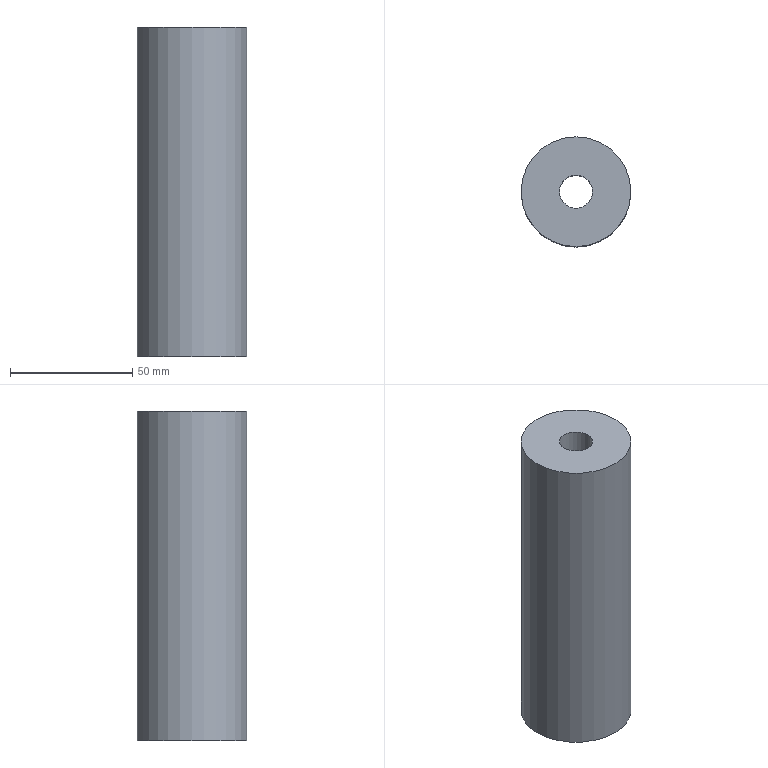Part | NX | features solid 2 | 1 solid | 6 faces | box 45 x 45 x 135.001 mm | volume 187665 mm3 | plane 3 | cylinder 3 | commonest cylinder face diameters 13.507 x1 20.008 x1 45 x1
STEP:
#1=CARTESIAN_POINT('',(1809.974,-158.405,-85.002));
#2=VERTEX_POINT('',#1);
#3=CARTESIAN_POINT('',(1819.978,-158.405,-85.002));
#4=DIRECTION('',(0.,0.,1.));
#5=DIRECTION('',(-1.,0.,0.));
#6=AXIS2_PLACEMENT_3D('',#3,#4,#5);
#7=CIRCLE('',#6,10.004);
#8=EDGE_CURVE('',#2,#2,#7,.T.);
#9=ORIENTED_EDGE('',*,*,#8,.T.);
#10=EDGE_LOOP('',(#9));
#11=FACE_BOUND('',#10,.T.);
#12=CARTESIAN_POINT('',(1842.478,-158.405,-85.002));
#13=VERTEX_POINT('',#12);
#14=CARTESIAN_POINT('',(1819.978,-158.405,-85.002));
#15=DIRECTION('',(0.,0.,-1.));
#16=DIRECTION('',(1.,0.,0.));
#17=AXIS2_PLACEMENT_3D('',#14,#15,#16);
#18=CIRCLE('',#17,22.5);
#19=EDGE_CURVE('',#13,#13,#18,.T.);
#20=ORIENTED_EDGE('',*,*,#19,.T.);
#21=EDGE_LOOP('',(#20));
#22=FACE_BOUND('',#21,.T.);
#23=CARTESIAN_POINT('',(2419.978,-148.405,-85.002));
#24=DIRECTION('',(0.,0.,-1.));
#25=DIRECTION('',(0.,-1.,0.));
#26=AXIS2_PLACEMENT_3D('',#23,#24,#25);
#27=PLANE('',#26);
#28=ADVANCED_FACE('',(#11,#22),#27,.T.);
#29=ORIENTED_EDGE('',*,*,#19,.F.);
#30=EDGE_LOOP('',(#29));
#31=FACE_BOUND('',#30,.T.);
#32=CARTESIAN_POINT('',(1842.478,-158.405,49.999));
#33=VERTEX_POINT('',#32);
#34=CARTESIAN_POINT('',(1819.978,-158.405,49.999));
#35=DIRECTION('',(0.,0.,-1.));
#36=DIRECTION('',(1.,0.,0.));
#37=AXIS2_PLACEMENT_3D('',#34,#35,#36);
#38=CIRCLE('',#37,22.5);
#39=EDGE_CURVE('',#33,#33,#38,.T.);
#40=ORIENTED_EDGE('',*,*,#39,.T.);
#41=EDGE_LOOP('',(#40));
#42=FACE_BOUND('',#41,.T.);
#43=CARTESIAN_POINT('',(1819.978,-158.405,-180.252));
#44=DIRECTION('',(0.,0.,-1.));
#45=DIRECTION('',(0.,-1.,0.));
#46=AXIS2_PLACEMENT_3D('',#43,#44,#45);
#47=CYLINDRICAL_SURFACE('',#46,22.5);
#48=ADVANCED_FACE('',(#31,#42),#47,.T.);
#49=CARTESIAN_POINT('',(1826.731,-158.405,49.999));
#50=VERTEX_POINT('',#49);
#51=CARTESIAN_POINT('',(1819.978,-158.405,49.999));
#52=DIRECTION('',(0.,0.,-1.));
#53=DIRECTION('',(1.,0.,0.));
#54=AXIS2_PLACEMENT_3D('',#51,#52,#53);
#55=CIRCLE('',#54,6.753);
#56=EDGE_CURVE('',#50,#50,#55,.T.);
#57=ORIENTED_EDGE('',*,*,#56,.T.);
#58=EDGE_LOOP('',(#57));
#59=FACE_BOUND('',#58,.T.);
#60=ORIENTED_EDGE('',*,*,#39,.F.);
#61=EDGE_LOOP('',(#60));
#62=FACE_BOUND('',#61,.T.);
#63=CARTESIAN_POINT('',(1541.955,75.94,49.999));
#64=DIRECTION('',(0.,0.,-1.));
#65=DIRECTION('',(-1.,0.,0.));
#66=AXIS2_PLACEMENT_3D('',#63,#64,#65);
#67=PLANE('',#66);
#68=ADVANCED_FACE('',(#59,#62),#67,.F.);
#69=ORIENTED_EDGE('',*,*,#8,.F.);
#70=EDGE_LOOP('',(#69));
#71=FACE_BOUND('',#70,.T.);
#72=CARTESIAN_POINT('',(1809.974,-158.405,-40.002));
#73=VERTEX_POINT('',#72);
#74=CARTESIAN_POINT('',(1819.978,-158.405,-40.002));
#75=DIRECTION('',(0.,0.,-1.));
#76=DIRECTION('',(-1.,0.,0.));
#77=AXIS2_PLACEMENT_3D('',#74,#75,#76);
#78=CIRCLE('',#77,10.004);
#79=EDGE_CURVE('',#73,#73,#78,.F.);
#80=ORIENTED_EDGE('',*,*,#79,.T.);
#81=EDGE_LOOP('',(#80));
#82=FACE_BOUND('',#81,.T.);
#83=CARTESIAN_POINT('',(1819.978,-158.405,-85.002));
#84=DIRECTION('',(0.,0.,1.));
#85=DIRECTION('',(-1.,0.,0.));
#86=AXIS2_PLACEMENT_3D('',#83,#84,#85);
#87=CYLINDRICAL_SURFACE('',#86,10.004);
#88=ADVANCED_FACE('',(#71,#82),#87,.F.);
#89=CARTESIAN_POINT('',(1826.731,-158.405,-40.002));
#90=VERTEX_POINT('',#89);
#91=CARTESIAN_POINT('',(1819.978,-158.405,-40.002));
#92=DIRECTION('',(0.,0.,1.));
#93=DIRECTION('',(1.,0.,0.));
#94=AXIS2_PLACEMENT_3D('',#91,#92,#93);
#95=CIRCLE('',#94,6.753);
#96=EDGE_CURVE('',#90,#90,#95,.T.);
#97=ORIENTED_EDGE('',*,*,#96,.F.);
#98=EDGE_LOOP('',(#97));
#99=FACE_BOUND('',#98,.T.);
#100=ORIENTED_EDGE('',*,*,#56,.F.);
#101=EDGE_LOOP('',(#100));
#102=FACE_BOUND('',#101,.T.);
#103=CARTESIAN_POINT('',(1819.978,-158.405,-215.002));
#104=DIRECTION('',(0.,0.,1.));
#105=DIRECTION('',(-1.,0.,0.));
#106=AXIS2_PLACEMENT_3D('',#103,#104,#105);
#107=CYLINDRICAL_SURFACE('',#106,6.753);
#108=ADVANCED_FACE('',(#99,#102),#107,.F.);
#109=ORIENTED_EDGE('',*,*,#96,.T.);
#110=EDGE_LOOP('',(#109));
#111=FACE_BOUND('',#110,.T.);
#112=ORIENTED_EDGE('',*,*,#79,.F.);
#113=EDGE_LOOP('',(#112));
#114=FACE_BOUND('',#113,.T.);
#115=CARTESIAN_POINT('',(1819.978,-158.405,-40.002));
#116=DIRECTION('',(0.,0.,1.));
#117=DIRECTION('',(1.,0.,0.));
#118=AXIS2_PLACEMENT_3D('',#115,#116,#117);
#119=PLANE('',#118);
#120=ADVANCED_FACE('',(#111,#114),#119,.F.);
#121=CLOSED_SHELL('',(#28,#48,#68,#88,#108,#120));
#122=MANIFOLD_SOLID_BREP('',#121);
#123=(LENGTH_UNIT()NAMED_UNIT(*)SI_UNIT(.MILLI.,.METRE.));
#124=UNCERTAINTY_MEASURE_WITH_UNIT(LENGTH_MEASURE(0.00001),#123,'','');
#125=(NAMED_UNIT(*)PLANE_ANGLE_UNIT()SI_UNIT($,.RADIAN.));
#126=(NAMED_UNIT(*)SI_UNIT($,.STERADIAN.)SOLID_ANGLE_UNIT());
#127=(GEOMETRIC_REPRESENTATION_CONTEXT(3)GLOBAL_UNCERTAINTY_ASSIGNED_CONTEXT((#124))GLOBAL_UNIT_ASSIGNED_CONTEXT((#123,#125,#126))REPRESENTATION_CONTEXT('',''));
#128=ADVANCED_BREP_SHAPE_REPRESENTATION('',(#122),#127);